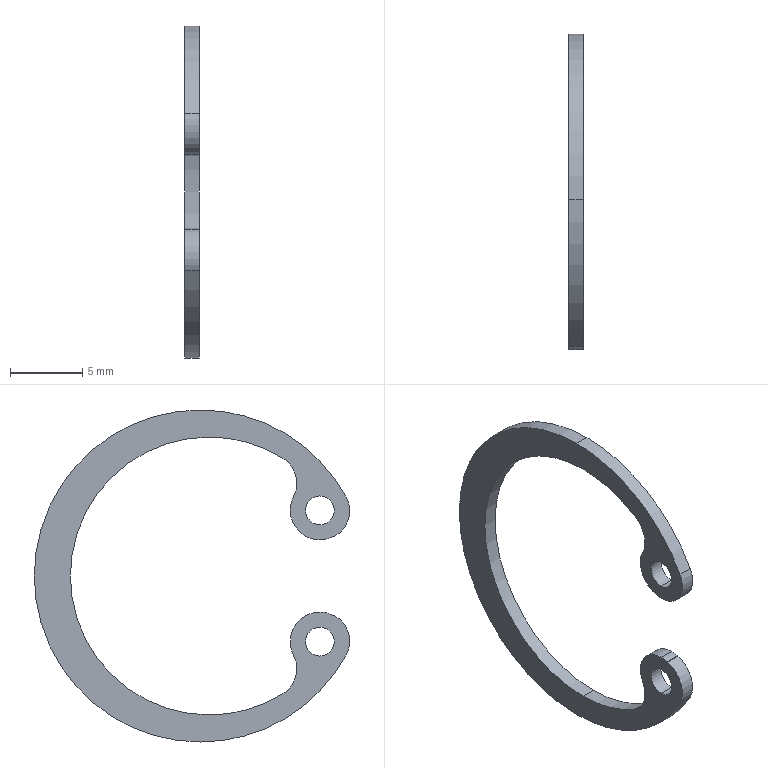Part | SolidWorks | features BaseBody 1 | 1 solid | 21 faces | box 1 x 21.856 x 23 mm | volume 128.626 mm3 | cylinder 17 | plane 4 | commonest cylinder face diameters 4.1 x5 2 x4 19.25 x3 23 x3 4 x2
STEP:
#1=CARTESIAN_POINT('',(-0.5,-8.916,-2.599));
#2=VERTEX_POINT('',#1);
#3=CARTESIAN_POINT('',(-0.5,-10.115,-5.471));
#4=VERTEX_POINT('',#3);
#5=CARTESIAN_POINT('',(-0.5,-8.356,-4.519));
#6=DIRECTION('',(1.,0.,0.));
#7=DIRECTION('',(0.,0.,-1.));
#8=AXIS2_PLACEMENT_3D('',#5,#6,#7);
#9=CIRCLE('',#8,2.);
#10=EDGE_CURVE('',#2,#4,#9,.T.);
#11=ORIENTED_EDGE('',*,*,#10,.T.);
#12=CARTESIAN_POINT('',(0.5,-10.115,-5.471));
#13=VERTEX_POINT('',#12);
#14=CARTESIAN_POINT('',(0.5,-10.115,-5.471));
#15=DIRECTION('',(-1.,0.,0.));
#16=VECTOR('',#15,1000.);
#17=LINE('',#14,#16);
#18=EDGE_CURVE('',#13,#4,#17,.T.);
#19=ORIENTED_EDGE('',*,*,#18,.F.);
#20=CARTESIAN_POINT('',(0.5,-8.916,-2.599));
#21=VERTEX_POINT('',#20);
#22=CARTESIAN_POINT('',(0.5,-8.356,-4.519));
#23=DIRECTION('',(1.,0.,0.));
#24=DIRECTION('',(0.,0.,-1.));
#25=AXIS2_PLACEMENT_3D('',#22,#23,#24);
#26=CIRCLE('',#25,2.);
#27=EDGE_CURVE('',#21,#13,#26,.T.);
#28=ORIENTED_EDGE('',*,*,#27,.F.);
#29=CARTESIAN_POINT('',(0.5,-8.916,-2.599));
#30=DIRECTION('',(-1.,0.,0.));
#31=VECTOR('',#30,1000.);
#32=LINE('',#29,#31);
#33=EDGE_CURVE('',#21,#2,#32,.T.);
#34=ORIENTED_EDGE('',*,*,#33,.T.);
#35=EDGE_LOOP('',(#11,#19,#28,#34));
#36=FACE_OUTER_BOUND('',#35,.T.);
#37=CARTESIAN_POINT('',(0.5,-8.356,-4.519));
#38=DIRECTION('',(-1.,0.,0.));
#39=DIRECTION('',(0.,0.,1.));
#40=AXIS2_PLACEMENT_3D('',#37,#38,#39);
#41=CYLINDRICAL_SURFACE('',#40,2.);
#42=ADVANCED_FACE('',(#36),#41,.T.);
#43=CARTESIAN_POINT('',(0.5,0.,-11.5));
#44=VERTEX_POINT('',#43);
#45=CARTESIAN_POINT('',(-0.5,0.,-11.5));
#46=VERTEX_POINT('',#45);
#47=CARTESIAN_POINT('',(0.5,0.,-11.5));
#48=DIRECTION('',(-1.,0.,0.));
#49=VECTOR('',#48,1000.);
#50=LINE('',#47,#49);
#51=EDGE_CURVE('',#44,#46,#50,.T.);
#52=ORIENTED_EDGE('',*,*,#51,.F.);
#53=CARTESIAN_POINT('',(0.5,0.,0.));
#54=DIRECTION('',(1.,0.,0.));
#55=DIRECTION('',(0.,0.,-1.));
#56=AXIS2_PLACEMENT_3D('',#53,#54,#55);
#57=CIRCLE('',#56,11.5);
#58=EDGE_CURVE('',#13,#44,#57,.T.);
#59=ORIENTED_EDGE('',*,*,#58,.F.);
#60=ORIENTED_EDGE('',*,*,#18,.T.);
#61=CARTESIAN_POINT('',(-0.5,0.,0.));
#62=DIRECTION('',(1.,0.,0.));
#63=DIRECTION('',(0.,0.,-1.));
#64=AXIS2_PLACEMENT_3D('',#61,#62,#63);
#65=CIRCLE('',#64,11.5);
#66=EDGE_CURVE('',#4,#46,#65,.T.);
#67=ORIENTED_EDGE('',*,*,#66,.T.);
#68=EDGE_LOOP('',(#52,#59,#60,#67));
#69=FACE_OUTER_BOUND('',#68,.T.);
#70=CARTESIAN_POINT('',(0.5,0.,0.));
#71=DIRECTION('',(-1.,0.,0.));
#72=DIRECTION('',(0.,0.,1.));
#73=AXIS2_PLACEMENT_3D('',#70,#71,#72);
#74=CYLINDRICAL_SURFACE('',#73,11.5);
#75=ADVANCED_FACE('',(#69),#74,.T.);
#76=CARTESIAN_POINT('',(-0.5,-10.115,5.471));
#77=VERTEX_POINT('',#76);
#78=CARTESIAN_POINT('',(-0.5,-8.916,2.599));
#79=VERTEX_POINT('',#78);
#80=CARTESIAN_POINT('',(-0.5,-8.356,4.519));
#81=DIRECTION('',(1.,0.,0.));
#82=DIRECTION('',(0.,0.,-1.));
#83=AXIS2_PLACEMENT_3D('',#80,#81,#82);
#84=CIRCLE('',#83,2.);
#85=EDGE_CURVE('',#77,#79,#84,.T.);
#86=ORIENTED_EDGE('',*,*,#85,.T.);
#87=CARTESIAN_POINT('',(0.5,-8.916,2.599));
#88=VERTEX_POINT('',#87);
#89=CARTESIAN_POINT('',(0.5,-8.916,2.599));
#90=DIRECTION('',(-1.,0.,0.));
#91=VECTOR('',#90,1000.);
#92=LINE('',#89,#91);
#93=EDGE_CURVE('',#88,#79,#92,.T.);
#94=ORIENTED_EDGE('',*,*,#93,.F.);
#95=CARTESIAN_POINT('',(0.5,-10.115,5.471));
#96=VERTEX_POINT('',#95);
#97=CARTESIAN_POINT('',(0.5,-8.356,4.519));
#98=DIRECTION('',(1.,0.,0.));
#99=DIRECTION('',(0.,0.,-1.));
#100=AXIS2_PLACEMENT_3D('',#97,#98,#99);
#101=CIRCLE('',#100,2.);
#102=EDGE_CURVE('',#96,#88,#101,.T.);
#103=ORIENTED_EDGE('',*,*,#102,.F.);
#104=CARTESIAN_POINT('',(0.5,-10.115,5.471));
#105=DIRECTION('',(-1.,0.,0.));
#106=VECTOR('',#105,1000.);
#107=LINE('',#104,#106);
#108=EDGE_CURVE('',#96,#77,#107,.T.);
#109=ORIENTED_EDGE('',*,*,#108,.T.);
#110=EDGE_LOOP('',(#86,#94,#103,#109));
#111=FACE_OUTER_BOUND('',#110,.T.);
#112=CARTESIAN_POINT('',(0.5,-8.356,4.519));
#113=DIRECTION('',(-1.,0.,0.));
#114=DIRECTION('',(0.,0.,1.));
#115=AXIS2_PLACEMENT_3D('',#112,#113,#114);
#116=CYLINDRICAL_SURFACE('',#115,2.);
#117=ADVANCED_FACE('',(#111),#116,.T.);
#118=CARTESIAN_POINT('',(-0.5,-8.856,2.582));
#119=VERTEX_POINT('',#118);
#120=CARTESIAN_POINT('',(-0.5,-8.916,2.599));
#121=DIRECTION('',(0.,0.96,-0.2799));
#122=VECTOR('',#121,1000.);
#123=LINE('',#120,#122);
#124=EDGE_CURVE('',#79,#119,#123,.T.);
#125=ORIENTED_EDGE('',*,*,#124,.T.);
#126=CARTESIAN_POINT('',(0.5,-8.856,2.582));
#127=VERTEX_POINT('',#126);
#128=CARTESIAN_POINT('',(0.5,-8.856,2.582));
#129=DIRECTION('',(-1.,0.,0.));
#130=VECTOR('',#129,1000.);
#131=LINE('',#128,#130);
#132=EDGE_CURVE('',#127,#119,#131,.T.);
#133=ORIENTED_EDGE('',*,*,#132,.F.);
#134=CARTESIAN_POINT('',(0.5,-8.916,2.599));
#135=DIRECTION('',(0.,0.96,-0.2799));
#136=VECTOR('',#135,1000.);
#137=LINE('',#134,#136);
#138=EDGE_CURVE('',#88,#127,#137,.T.);
#139=ORIENTED_EDGE('',*,*,#138,.F.);
#140=ORIENTED_EDGE('',*,*,#93,.T.);
#141=EDGE_LOOP('',(#125,#133,#139,#140));
#142=FACE_OUTER_BOUND('',#141,.T.);
#143=CARTESIAN_POINT('',(0.5,-8.916,2.599));
#144=DIRECTION('',(0.,0.2799,0.96));
#145=DIRECTION('',(1.,0.,0.));
#146=AXIS2_PLACEMENT_3D('',#143,#144,#145);
#147=PLANE('',#146);
#148=ADVANCED_FACE('',(#142),#147,.F.);
#149=CARTESIAN_POINT('',(-0.5,-6.46,5.488));
#150=VERTEX_POINT('',#149);
#151=CARTESIAN_POINT('',(-0.5,-8.283,4.55));
#152=DIRECTION('',(1.,0.,0.));
#153=DIRECTION('',(0.,0.,-1.));
#154=AXIS2_PLACEMENT_3D('',#151,#152,#153);
#155=CIRCLE('',#154,2.05);
#156=EDGE_CURVE('',#119,#150,#155,.T.);
#157=ORIENTED_EDGE('',*,*,#156,.T.);
#158=CARTESIAN_POINT('',(0.5,-6.46,5.488));
#159=VERTEX_POINT('',#158);
#160=CARTESIAN_POINT('',(0.5,-6.46,5.488));
#161=DIRECTION('',(-1.,0.,0.));
#162=VECTOR('',#161,1000.);
#163=LINE('',#160,#162);
#164=EDGE_CURVE('',#159,#150,#163,.T.);
#165=ORIENTED_EDGE('',*,*,#164,.F.);
#166=CARTESIAN_POINT('',(0.5,-8.283,4.55));
#167=DIRECTION('',(1.,0.,0.));
#168=DIRECTION('',(0.,0.,-1.));
#169=AXIS2_PLACEMENT_3D('',#166,#167,#168);
#170=CIRCLE('',#169,2.05);
#171=EDGE_CURVE('',#127,#159,#170,.T.);
#172=ORIENTED_EDGE('',*,*,#171,.F.);
#173=ORIENTED_EDGE('',*,*,#132,.T.);
#174=EDGE_LOOP('',(#157,#165,#172,#173));
#175=FACE_OUTER_BOUND('',#174,.T.);
#176=CARTESIAN_POINT('',(0.5,-8.283,4.55));
#177=DIRECTION('',(-1.,0.,0.));
#178=DIRECTION('',(0.,0.,1.));
#179=AXIS2_PLACEMENT_3D('',#176,#177,#178);
#180=CYLINDRICAL_SURFACE('',#179,2.05);
#181=ADVANCED_FACE('',(#175),#180,.T.);
#182=CARTESIAN_POINT('',(-0.5,-5.722,8.164));
#183=VERTEX_POINT('',#182);
#184=CARTESIAN_POINT('',(-0.5,-4.637,6.426));
#185=DIRECTION('',(1.,0.,0.));
#186=DIRECTION('',(0.,0.,-1.));
#187=AXIS2_PLACEMENT_3D('',#184,#185,#186);
#188=CIRCLE('',#187,2.05);
#189=EDGE_CURVE('',#183,#150,#188,.T.);
#190=ORIENTED_EDGE('',*,*,#189,.F.);
#191=CARTESIAN_POINT('',(0.5,-5.722,8.164));
#192=VERTEX_POINT('',#191);
#193=CARTESIAN_POINT('',(0.5,-5.722,8.164));
#194=DIRECTION('',(-1.,0.,0.));
#195=VECTOR('',#194,1000.);
#196=LINE('',#193,#195);
#197=EDGE_CURVE('',#192,#183,#196,.T.);
#198=ORIENTED_EDGE('',*,*,#197,.F.);
#199=CARTESIAN_POINT('',(0.5,-4.637,6.426));
#200=DIRECTION('',(1.,0.,0.));
#201=DIRECTION('',(0.,0.,-1.));
#202=AXIS2_PLACEMENT_3D('',#199,#200,#201);
#203=CIRCLE('',#202,2.05);
#204=EDGE_CURVE('',#192,#159,#203,.T.);
#205=ORIENTED_EDGE('',*,*,#204,.T.);
#206=ORIENTED_EDGE('',*,*,#164,.T.);
#207=EDGE_LOOP('',(#190,#198,#205,#206));
#208=FACE_OUTER_BOUND('',#207,.T.);
#209=CARTESIAN_POINT('',(0.5,-4.637,6.426));
#210=DIRECTION('',(-1.,0.,0.));
#211=DIRECTION('',(0.,0.,1.));
#212=AXIS2_PLACEMENT_3D('',#209,#210,#211);
#213=CYLINDRICAL_SURFACE('',#212,2.05);
#214=ADVANCED_FACE('',(#208),#213,.F.);
#215=CARTESIAN_POINT('',(0.5,-0.625,9.625));
#216=VERTEX_POINT('',#215);
#217=CARTESIAN_POINT('',(-0.5,-0.625,9.625));
#218=VERTEX_POINT('',#217);
#219=CARTESIAN_POINT('',(0.5,-0.625,9.625));
#220=DIRECTION('',(-1.,0.,0.));
#221=VECTOR('',#220,1000.);
#222=LINE('',#219,#221);
#223=EDGE_CURVE('',#216,#218,#222,.T.);
#224=ORIENTED_EDGE('',*,*,#223,.F.);
#225=CARTESIAN_POINT('',(0.5,-0.625,0.));
#226=DIRECTION('',(1.,0.,0.));
#227=DIRECTION('',(0.,0.,-1.));
#228=AXIS2_PLACEMENT_3D('',#225,#226,#227);
#229=CIRCLE('',#228,9.625);
#230=EDGE_CURVE('',#216,#192,#229,.T.);
#231=ORIENTED_EDGE('',*,*,#230,.T.);
#232=ORIENTED_EDGE('',*,*,#197,.T.);
#233=CARTESIAN_POINT('',(-0.5,-0.625,0.));
#234=DIRECTION('',(1.,0.,0.));
#235=DIRECTION('',(0.,0.,-1.));
#236=AXIS2_PLACEMENT_3D('',#233,#234,#235);
#237=CIRCLE('',#236,9.625);
#238=EDGE_CURVE('',#218,#183,#237,.T.);
#239=ORIENTED_EDGE('',*,*,#238,.F.);
#240=EDGE_LOOP('',(#224,#231,#232,#239));
#241=FACE_OUTER_BOUND('',#240,.T.);
#242=CARTESIAN_POINT('',(0.5,-0.625,0.));
#243=DIRECTION('',(-1.,0.,0.));
#244=DIRECTION('',(0.,0.,1.));
#245=AXIS2_PLACEMENT_3D('',#242,#243,#244);
#246=CYLINDRICAL_SURFACE('',#245,9.625);
#247=ADVANCED_FACE('',(#241),#246,.F.);
#248=CARTESIAN_POINT('',(-0.5,-6.46,-5.488));
#249=VERTEX_POINT('',#248);
#250=CARTESIAN_POINT('',(-0.5,-5.722,-8.164));
#251=VERTEX_POINT('',#250);
#252=CARTESIAN_POINT('',(-0.5,-4.637,-6.426));
#253=DIRECTION('',(1.,0.,0.));
#254=DIRECTION('',(0.,0.,-1.));
#255=AXIS2_PLACEMENT_3D('',#252,#253,#254);
#256=CIRCLE('',#255,2.05);
#257=EDGE_CURVE('',#249,#251,#256,.T.);
#258=ORIENTED_EDGE('',*,*,#257,.F.);
#259=CARTESIAN_POINT('',(0.5,-6.46,-5.488));
#260=VERTEX_POINT('',#259);
#261=CARTESIAN_POINT('',(0.5,-6.46,-5.488));
#262=DIRECTION('',(-1.,0.,0.));
#263=VECTOR('',#262,1000.);
#264=LINE('',#261,#263);
#265=EDGE_CURVE('',#260,#249,#264,.T.);
#266=ORIENTED_EDGE('',*,*,#265,.F.);
#267=CARTESIAN_POINT('',(0.5,-5.722,-8.164));
#268=VERTEX_POINT('',#267);
#269=CARTESIAN_POINT('',(0.5,-4.637,-6.426));
#270=DIRECTION('',(1.,0.,0.));
#271=DIRECTION('',(0.,0.,-1.));
#272=AXIS2_PLACEMENT_3D('',#269,#270,#271);
#273=CIRCLE('',#272,2.05);
#274=EDGE_CURVE('',#260,#268,#273,.T.);
#275=ORIENTED_EDGE('',*,*,#274,.T.);
#276=CARTESIAN_POINT('',(0.5,-5.722,-8.164));
#277=DIRECTION('',(-1.,0.,0.));
#278=VECTOR('',#277,1000.);
#279=LINE('',#276,#278);
#280=EDGE_CURVE('',#268,#251,#279,.T.);
#281=ORIENTED_EDGE('',*,*,#280,.T.);
#282=EDGE_LOOP('',(#258,#266,#275,#281));
#283=FACE_OUTER_BOUND('',#282,.T.);
#284=CARTESIAN_POINT('',(0.5,-4.637,-6.426));
#285=DIRECTION('',(-1.,0.,0.));
#286=DIRECTION('',(0.,0.,1.));
#287=AXIS2_PLACEMENT_3D('',#284,#285,#286);
#288=CYLINDRICAL_SURFACE('',#287,2.05);
#289=ADVANCED_FACE('',(#283),#288,.F.);
#290=CARTESIAN_POINT('',(0.5,-8.283,-2.5));
#291=VERTEX_POINT('',#290);
#292=CARTESIAN_POINT('',(-0.5,-8.283,-2.5));
#293=VERTEX_POINT('',#292);
#294=CARTESIAN_POINT('',(0.5,-8.283,-2.5));
#295=DIRECTION('',(-1.,0.,0.));
#296=VECTOR('',#295,1000.);
#297=LINE('',#294,#296);
#298=EDGE_CURVE('',#291,#293,#297,.T.);
#299=ORIENTED_EDGE('',*,*,#298,.F.);
#300=CARTESIAN_POINT('',(0.5,-8.283,-4.55));
#301=DIRECTION('',(1.,0.,0.));
#302=DIRECTION('',(0.,0.,-1.));
#303=AXIS2_PLACEMENT_3D('',#300,#301,#302);
#304=CIRCLE('',#303,2.05);
#305=EDGE_CURVE('',#260,#291,#304,.T.);
#306=ORIENTED_EDGE('',*,*,#305,.F.);
#307=ORIENTED_EDGE('',*,*,#265,.T.);
#308=CARTESIAN_POINT('',(-0.5,-8.283,-4.55));
#309=DIRECTION('',(1.,0.,0.));
#310=DIRECTION('',(0.,0.,-1.));
#311=AXIS2_PLACEMENT_3D('',#308,#309,#310);
#312=CIRCLE('',#311,2.05);
#313=EDGE_CURVE('',#249,#293,#312,.T.);
#314=ORIENTED_EDGE('',*,*,#313,.T.);
#315=EDGE_LOOP('',(#299,#306,#307,#314));
#316=FACE_OUTER_BOUND('',#315,.T.);
#317=CARTESIAN_POINT('',(0.5,-8.283,-4.55));
#318=DIRECTION('',(-1.,0.,0.));
#319=DIRECTION('',(0.,0.,1.));
#320=AXIS2_PLACEMENT_3D('',#317,#318,#319);
#321=CYLINDRICAL_SURFACE('',#320,2.05);
#322=ADVANCED_FACE('',(#316),#321,.T.);
#323=CARTESIAN_POINT('',(0.5,-8.283,-5.55));
#324=VERTEX_POINT('',#323);
#325=CARTESIAN_POINT('',(-0.5,-8.283,-5.55));
#326=VERTEX_POINT('',#325);
#327=CARTESIAN_POINT('',(0.5,-8.283,-5.55));
#328=DIRECTION('',(-1.,0.,0.));
#329=VECTOR('',#328,1000.);
#330=LINE('',#327,#329);
#331=EDGE_CURVE('',#324,#326,#330,.T.);
#332=ORIENTED_EDGE('',*,*,#331,.F.);
#333=CARTESIAN_POINT('',(0.5,-8.283,-3.55));
#334=VERTEX_POINT('',#333);
#335=CARTESIAN_POINT('',(0.5,-8.283,-4.55));
#336=DIRECTION('',(1.,0.,0.));
#337=DIRECTION('',(0.,0.,-1.));
#338=AXIS2_PLACEMENT_3D('',#335,#336,#337);
#339=CIRCLE('',#338,1.);
#340=EDGE_CURVE('',#324,#334,#339,.T.);
#341=ORIENTED_EDGE('',*,*,#340,.T.);
#342=CARTESIAN_POINT('',(-0.5,-8.283,-3.55));
#343=VERTEX_POINT('',#342);
#344=CARTESIAN_POINT('',(0.5,-8.283,-3.55));
#345=DIRECTION('',(-1.,0.,0.));
#346=VECTOR('',#345,1000.);
#347=LINE('',#344,#346);
#348=EDGE_CURVE('',#334,#343,#347,.T.);
#349=ORIENTED_EDGE('',*,*,#348,.T.);
#350=CARTESIAN_POINT('',(-0.5,-8.283,-4.55));
#351=DIRECTION('',(1.,0.,0.));
#352=DIRECTION('',(0.,0.,-1.));
#353=AXIS2_PLACEMENT_3D('',#350,#351,#352);
#354=CIRCLE('',#353,1.);
#355=EDGE_CURVE('',#326,#343,#354,.T.);
#356=ORIENTED_EDGE('',*,*,#355,.F.);
#357=EDGE_LOOP('',(#332,#341,#349,#356));
#358=FACE_OUTER_BOUND('',#357,.T.);
#359=CARTESIAN_POINT('',(0.5,-8.283,-4.55));
#360=DIRECTION('',(-1.,0.,0.));
#361=DIRECTION('',(0.,0.,1.));
#362=AXIS2_PLACEMENT_3D('',#359,#360,#361);
#363=CYLINDRICAL_SURFACE('',#362,1.);
#364=ADVANCED_FACE('',(#358),#363,.F.);
#365=CARTESIAN_POINT('',(0.5,-8.283,3.55));
#366=VERTEX_POINT('',#365);
#367=CARTESIAN_POINT('',(-0.5,-8.283,3.55));
#368=VERTEX_POINT('',#367);
#369=CARTESIAN_POINT('',(0.5,-8.283,3.55));
#370=DIRECTION('',(-1.,0.,0.));
#371=VECTOR('',#370,1000.);
#372=LINE('',#369,#371);
#373=EDGE_CURVE('',#366,#368,#372,.T.);
#374=ORIENTED_EDGE('',*,*,#373,.F.);
#375=CARTESIAN_POINT('',(0.5,-8.283,5.55));
#376=VERTEX_POINT('',#375);
#377=CARTESIAN_POINT('',(0.5,-8.283,4.55));
#378=DIRECTION('',(1.,0.,0.));
#379=DIRECTION('',(0.,0.,-1.));
#380=AXIS2_PLACEMENT_3D('',#377,#378,#379);
#381=CIRCLE('',#380,1.);
#382=EDGE_CURVE('',#366,#376,#381,.T.);
#383=ORIENTED_EDGE('',*,*,#382,.T.);
#384=CARTESIAN_POINT('',(-0.5,-8.283,5.55));
#385=VERTEX_POINT('',#384);
#386=CARTESIAN_POINT('',(0.5,-8.283,5.55));
#387=DIRECTION('',(-1.,0.,0.));
#388=VECTOR('',#387,1000.);
#389=LINE('',#386,#388);
#390=EDGE_CURVE('',#376,#385,#389,.T.);
#391=ORIENTED_EDGE('',*,*,#390,.T.);
#392=CARTESIAN_POINT('',(-0.5,-8.283,4.55));
#393=DIRECTION('',(1.,0.,0.));
#394=DIRECTION('',(0.,0.,-1.));
#395=AXIS2_PLACEMENT_3D('',#392,#393,#394);
#396=CIRCLE('',#395,1.);
#397=EDGE_CURVE('',#368,#385,#396,.T.);
#398=ORIENTED_EDGE('',*,*,#397,.F.);
#399=EDGE_LOOP('',(#374,#383,#391,#398));
#400=FACE_OUTER_BOUND('',#399,.T.);
#401=CARTESIAN_POINT('',(0.5,-8.283,4.55));
#402=DIRECTION('',(-1.,0.,0.));
#403=DIRECTION('',(0.,0.,1.));
#404=AXIS2_PLACEMENT_3D('',#401,#402,#403);
#405=CYLINDRICAL_SURFACE('',#404,1.);
#406=ADVANCED_FACE('',(#400),#405,.F.);
#407=CARTESIAN_POINT('',(-0.5,-8.856,-2.582));
#408=VERTEX_POINT('',#407);
#409=CARTESIAN_POINT('',(-0.5,-8.856,-2.582));
#410=DIRECTION('',(0.,-0.96,-0.2799));
#411=VECTOR('',#410,1000.);
#412=LINE('',#409,#411);
#413=EDGE_CURVE('',#408,#2,#412,.T.);
#414=ORIENTED_EDGE('',*,*,#413,.T.);
#415=ORIENTED_EDGE('',*,*,#33,.F.);
#416=CARTESIAN_POINT('',(0.5,-8.856,-2.582));
#417=VERTEX_POINT('',#416);
#418=CARTESIAN_POINT('',(0.5,-8.856,-2.582));
#419=DIRECTION('',(0.,-0.96,-0.2799));
#420=VECTOR('',#419,1000.);
#421=LINE('',#418,#420);
#422=EDGE_CURVE('',#417,#21,#421,.T.);
#423=ORIENTED_EDGE('',*,*,#422,.F.);
#424=CARTESIAN_POINT('',(0.5,-8.856,-2.582));
#425=DIRECTION('',(-1.,0.,0.));
#426=VECTOR('',#425,1000.);
#427=LINE('',#424,#426);
#428=EDGE_CURVE('',#417,#408,#427,.T.);
#429=ORIENTED_EDGE('',*,*,#428,.T.);
#430=EDGE_LOOP('',(#414,#415,#423,#429));
#431=FACE_OUTER_BOUND('',#430,.T.);
#432=CARTESIAN_POINT('',(0.5,-8.856,-2.582));
#433=DIRECTION('',(0.,0.2799,-0.96));
#434=DIRECTION('',(-1.,0.,0.));
#435=AXIS2_PLACEMENT_3D('',#432,#433,#434);
#436=PLANE('',#435);
#437=ADVANCED_FACE('',(#431),#436,.F.);
#438=CARTESIAN_POINT('',(0.5,-8.283,4.55));
#439=DIRECTION('',(1.,0.,0.));
#440=DIRECTION('',(0.,0.,-1.));
#441=AXIS2_PLACEMENT_3D('',#438,#439,#440);
#442=CIRCLE('',#441,1.);
#443=EDGE_CURVE('',#376,#366,#442,.T.);
#444=ORIENTED_EDGE('',*,*,#443,.F.);
#445=ORIENTED_EDGE('',*,*,#382,.F.);
#446=EDGE_LOOP('',(#444,#445));
#447=FACE_BOUND('',#446,.T.);
#448=CARTESIAN_POINT('',(0.5,-8.283,-4.55));
#449=DIRECTION('',(1.,0.,0.));
#450=DIRECTION('',(0.,0.,-1.));
#451=AXIS2_PLACEMENT_3D('',#448,#449,#450);
#452=CIRCLE('',#451,1.);
#453=EDGE_CURVE('',#334,#324,#452,.T.);
#454=ORIENTED_EDGE('',*,*,#453,.F.);
#455=ORIENTED_EDGE('',*,*,#340,.F.);
#456=EDGE_LOOP('',(#454,#455));
#457=FACE_BOUND('',#456,.T.);
#458=ORIENTED_EDGE('',*,*,#27,.T.);
#459=ORIENTED_EDGE('',*,*,#58,.T.);
#460=CARTESIAN_POINT('',(0.5,0.,11.5));
#461=VERTEX_POINT('',#460);
#462=CARTESIAN_POINT('',(0.5,0.,0.));
#463=DIRECTION('',(1.,0.,0.));
#464=DIRECTION('',(0.,0.,-1.));
#465=AXIS2_PLACEMENT_3D('',#462,#463,#464);
#466=CIRCLE('',#465,11.5);
#467=EDGE_CURVE('',#44,#461,#466,.T.);
#468=ORIENTED_EDGE('',*,*,#467,.T.);
#469=CARTESIAN_POINT('',(0.5,0.,0.));
#470=DIRECTION('',(1.,0.,0.));
#471=DIRECTION('',(0.,0.,-1.));
#472=AXIS2_PLACEMENT_3D('',#469,#470,#471);
#473=CIRCLE('',#472,11.5);
#474=EDGE_CURVE('',#461,#96,#473,.T.);
#475=ORIENTED_EDGE('',*,*,#474,.T.);
#476=ORIENTED_EDGE('',*,*,#102,.T.);
#477=ORIENTED_EDGE('',*,*,#138,.T.);
#478=ORIENTED_EDGE('',*,*,#171,.T.);
#479=ORIENTED_EDGE('',*,*,#204,.F.);
#480=ORIENTED_EDGE('',*,*,#230,.F.);
#481=CARTESIAN_POINT('',(0.5,-0.625,-9.625));
#482=VERTEX_POINT('',#481);
#483=CARTESIAN_POINT('',(0.5,-0.625,0.));
#484=DIRECTION('',(1.,0.,0.));
#485=DIRECTION('',(0.,0.,-1.));
#486=AXIS2_PLACEMENT_3D('',#483,#484,#485);
#487=CIRCLE('',#486,9.625);
#488=EDGE_CURVE('',#482,#216,#487,.T.);
#489=ORIENTED_EDGE('',*,*,#488,.F.);
#490=CARTESIAN_POINT('',(0.5,-0.625,0.));
#491=DIRECTION('',(1.,0.,0.));
#492=DIRECTION('',(0.,0.,-1.));
#493=AXIS2_PLACEMENT_3D('',#490,#491,#492);
#494=CIRCLE('',#493,9.625);
#495=EDGE_CURVE('',#268,#482,#494,.T.);
#496=ORIENTED_EDGE('',*,*,#495,.F.);
#497=ORIENTED_EDGE('',*,*,#274,.F.);
#498=ORIENTED_EDGE('',*,*,#305,.T.);
#499=CARTESIAN_POINT('',(0.5,-8.283,-4.55));
#500=DIRECTION('',(1.,0.,0.));
#501=DIRECTION('',(0.,0.,-1.));
#502=AXIS2_PLACEMENT_3D('',#499,#500,#501);
#503=CIRCLE('',#502,2.05);
#504=EDGE_CURVE('',#291,#417,#503,.T.);
#505=ORIENTED_EDGE('',*,*,#504,.T.);
#506=ORIENTED_EDGE('',*,*,#422,.T.);
#507=EDGE_LOOP('',(#458,#459,#468,#475,#476,#477,#478,#479,#480,#489,#496,#497,#498,#505,#506));
#508=FACE_OUTER_BOUND('',#507,.T.);
#509=CARTESIAN_POINT('',(0.5,-8.356,-4.519));
#510=DIRECTION('',(1.,0.,0.));
#511=DIRECTION('',(0.,1.,0.));
#512=AXIS2_PLACEMENT_3D('',#509,#510,#511);
#513=PLANE('',#512);
#514=ADVANCED_FACE('',(#447,#457,#508),#513,.T.);
#515=CARTESIAN_POINT('',(-0.5,-8.283,4.55));
#516=DIRECTION('',(1.,0.,0.));
#517=DIRECTION('',(0.,0.,-1.));
#518=AXIS2_PLACEMENT_3D('',#515,#516,#517);
#519=CIRCLE('',#518,1.);
#520=EDGE_CURVE('',#385,#368,#519,.T.);
#521=ORIENTED_EDGE('',*,*,#520,.T.);
#522=ORIENTED_EDGE('',*,*,#397,.T.);
#523=EDGE_LOOP('',(#521,#522));
#524=FACE_BOUND('',#523,.T.);
#525=CARTESIAN_POINT('',(-0.5,-8.283,-4.55));
#526=DIRECTION('',(1.,0.,0.));
#527=DIRECTION('',(0.,0.,-1.));
#528=AXIS2_PLACEMENT_3D('',#525,#526,#527);
#529=CIRCLE('',#528,1.);
#530=EDGE_CURVE('',#343,#326,#529,.T.);
#531=ORIENTED_EDGE('',*,*,#530,.T.);
#532=ORIENTED_EDGE('',*,*,#355,.T.);
#533=EDGE_LOOP('',(#531,#532));
#534=FACE_BOUND('',#533,.T.);
#535=ORIENTED_EDGE('',*,*,#10,.F.);
#536=ORIENTED_EDGE('',*,*,#413,.F.);
#537=CARTESIAN_POINT('',(-0.5,-8.283,-4.55));
#538=DIRECTION('',(1.,0.,0.));
#539=DIRECTION('',(0.,0.,-1.));
#540=AXIS2_PLACEMENT_3D('',#537,#538,#539);
#541=CIRCLE('',#540,2.05);
#542=EDGE_CURVE('',#293,#408,#541,.T.);
#543=ORIENTED_EDGE('',*,*,#542,.F.);
#544=ORIENTED_EDGE('',*,*,#313,.F.);
#545=ORIENTED_EDGE('',*,*,#257,.T.);
#546=CARTESIAN_POINT('',(-0.5,-0.625,-9.625));
#547=VERTEX_POINT('',#546);
#548=CARTESIAN_POINT('',(-0.5,-0.625,0.));
#549=DIRECTION('',(1.,0.,0.));
#550=DIRECTION('',(0.,0.,-1.));
#551=AXIS2_PLACEMENT_3D('',#548,#549,#550);
#552=CIRCLE('',#551,9.625);
#553=EDGE_CURVE('',#251,#547,#552,.T.);
#554=ORIENTED_EDGE('',*,*,#553,.T.);
#555=CARTESIAN_POINT('',(-0.5,-0.625,0.));
#556=DIRECTION('',(1.,0.,0.));
#557=DIRECTION('',(0.,0.,-1.));
#558=AXIS2_PLACEMENT_3D('',#555,#556,#557);
#559=CIRCLE('',#558,9.625);
#560=EDGE_CURVE('',#547,#218,#559,.T.);
#561=ORIENTED_EDGE('',*,*,#560,.T.);
#562=ORIENTED_EDGE('',*,*,#238,.T.);
#563=ORIENTED_EDGE('',*,*,#189,.T.);
#564=ORIENTED_EDGE('',*,*,#156,.F.);
#565=ORIENTED_EDGE('',*,*,#124,.F.);
#566=ORIENTED_EDGE('',*,*,#85,.F.);
#567=CARTESIAN_POINT('',(-0.5,0.,11.5));
#568=VERTEX_POINT('',#567);
#569=CARTESIAN_POINT('',(-0.5,0.,0.));
#570=DIRECTION('',(1.,0.,0.));
#571=DIRECTION('',(0.,0.,-1.));
#572=AXIS2_PLACEMENT_3D('',#569,#570,#571);
#573=CIRCLE('',#572,11.5);
#574=EDGE_CURVE('',#568,#77,#573,.T.);
#575=ORIENTED_EDGE('',*,*,#574,.F.);
#576=CARTESIAN_POINT('',(-0.5,0.,0.));
#577=DIRECTION('',(1.,0.,0.));
#578=DIRECTION('',(0.,0.,-1.));
#579=AXIS2_PLACEMENT_3D('',#576,#577,#578);
#580=CIRCLE('',#579,11.5);
#581=EDGE_CURVE('',#46,#568,#580,.T.);
#582=ORIENTED_EDGE('',*,*,#581,.F.);
#583=ORIENTED_EDGE('',*,*,#66,.F.);
#584=EDGE_LOOP('',(#535,#536,#543,#544,#545,#554,#561,#562,#563,#564,#565,#566,#575,#582,#583));
#585=FACE_OUTER_BOUND('',#584,.T.);
#586=CARTESIAN_POINT('',(-0.5,-8.356,-4.519));
#587=DIRECTION('',(1.,0.,0.));
#588=DIRECTION('',(0.,1.,0.));
#589=AXIS2_PLACEMENT_3D('',#586,#587,#588);
#590=PLANE('',#589);
#591=ADVANCED_FACE('',(#524,#534,#585),#590,.F.);
#592=ORIENTED_EDGE('',*,*,#443,.T.);
#593=ORIENTED_EDGE('',*,*,#373,.T.);
#594=ORIENTED_EDGE('',*,*,#520,.F.);
#595=ORIENTED_EDGE('',*,*,#390,.F.);
#596=EDGE_LOOP('',(#592,#593,#594,#595));
#597=FACE_OUTER_BOUND('',#596,.T.);
#598=CARTESIAN_POINT('',(0.5,-8.283,4.55));
#599=DIRECTION('',(-1.,0.,0.));
#600=DIRECTION('',(0.,0.,1.));
#601=AXIS2_PLACEMENT_3D('',#598,#599,#600);
#602=CYLINDRICAL_SURFACE('',#601,1.);
#603=ADVANCED_FACE('',(#597),#602,.F.);
#604=ORIENTED_EDGE('',*,*,#453,.T.);
#605=ORIENTED_EDGE('',*,*,#331,.T.);
#606=ORIENTED_EDGE('',*,*,#530,.F.);
#607=ORIENTED_EDGE('',*,*,#348,.F.);
#608=EDGE_LOOP('',(#604,#605,#606,#607));
#609=FACE_OUTER_BOUND('',#608,.T.);
#610=CARTESIAN_POINT('',(0.5,-8.283,-4.55));
#611=DIRECTION('',(-1.,0.,0.));
#612=DIRECTION('',(0.,0.,1.));
#613=AXIS2_PLACEMENT_3D('',#610,#611,#612);
#614=CYLINDRICAL_SURFACE('',#613,1.);
#615=ADVANCED_FACE('',(#609),#614,.F.);
#616=ORIENTED_EDGE('',*,*,#504,.F.);
#617=ORIENTED_EDGE('',*,*,#298,.T.);
#618=ORIENTED_EDGE('',*,*,#542,.T.);
#619=ORIENTED_EDGE('',*,*,#428,.F.);
#620=EDGE_LOOP('',(#616,#617,#618,#619));
#621=FACE_OUTER_BOUND('',#620,.T.);
#622=CARTESIAN_POINT('',(0.5,-8.283,-4.55));
#623=DIRECTION('',(-1.,0.,0.));
#624=DIRECTION('',(0.,0.,1.));
#625=AXIS2_PLACEMENT_3D('',#622,#623,#624);
#626=CYLINDRICAL_SURFACE('',#625,2.05);
#627=ADVANCED_FACE('',(#621),#626,.T.);
#628=CARTESIAN_POINT('',(0.5,-0.625,-9.625));
#629=DIRECTION('',(-1.,0.,0.));
#630=VECTOR('',#629,1000.);
#631=LINE('',#628,#630);
#632=EDGE_CURVE('',#482,#547,#631,.T.);
#633=ORIENTED_EDGE('',*,*,#632,.F.);
#634=ORIENTED_EDGE('',*,*,#488,.T.);
#635=ORIENTED_EDGE('',*,*,#223,.T.);
#636=ORIENTED_EDGE('',*,*,#560,.F.);
#637=EDGE_LOOP('',(#633,#634,#635,#636));
#638=FACE_OUTER_BOUND('',#637,.T.);
#639=CARTESIAN_POINT('',(0.5,-0.625,0.));
#640=DIRECTION('',(-1.,0.,0.));
#641=DIRECTION('',(0.,0.,1.));
#642=AXIS2_PLACEMENT_3D('',#639,#640,#641);
#643=CYLINDRICAL_SURFACE('',#642,9.625);
#644=ADVANCED_FACE('',(#638),#643,.F.);
#645=ORIENTED_EDGE('',*,*,#495,.T.);
#646=ORIENTED_EDGE('',*,*,#632,.T.);
#647=ORIENTED_EDGE('',*,*,#553,.F.);
#648=ORIENTED_EDGE('',*,*,#280,.F.);
#649=EDGE_LOOP('',(#645,#646,#647,#648));
#650=FACE_OUTER_BOUND('',#649,.T.);
#651=CARTESIAN_POINT('',(0.5,-0.625,0.));
#652=DIRECTION('',(-1.,0.,0.));
#653=DIRECTION('',(0.,0.,1.));
#654=AXIS2_PLACEMENT_3D('',#651,#652,#653);
#655=CYLINDRICAL_SURFACE('',#654,9.625);
#656=ADVANCED_FACE('',(#650),#655,.F.);
#657=ORIENTED_EDGE('',*,*,#474,.F.);
#658=CARTESIAN_POINT('',(0.5,0.,11.5));
#659=DIRECTION('',(-1.,0.,0.));
#660=VECTOR('',#659,1000.);
#661=LINE('',#658,#660);
#662=EDGE_CURVE('',#461,#568,#661,.T.);
#663=ORIENTED_EDGE('',*,*,#662,.T.);
#664=ORIENTED_EDGE('',*,*,#574,.T.);
#665=ORIENTED_EDGE('',*,*,#108,.F.);
#666=EDGE_LOOP('',(#657,#663,#664,#665));
#667=FACE_OUTER_BOUND('',#666,.T.);
#668=CARTESIAN_POINT('',(0.5,0.,0.));
#669=DIRECTION('',(-1.,0.,0.));
#670=DIRECTION('',(0.,0.,1.));
#671=AXIS2_PLACEMENT_3D('',#668,#669,#670);
#672=CYLINDRICAL_SURFACE('',#671,11.5);
#673=ADVANCED_FACE('',(#667),#672,.T.);
#674=ORIENTED_EDGE('',*,*,#467,.F.);
#675=ORIENTED_EDGE('',*,*,#51,.T.);
#676=ORIENTED_EDGE('',*,*,#581,.T.);
#677=ORIENTED_EDGE('',*,*,#662,.F.);
#678=EDGE_LOOP('',(#674,#675,#676,#677));
#679=FACE_OUTER_BOUND('',#678,.T.);
#680=CARTESIAN_POINT('',(0.5,0.,0.));
#681=DIRECTION('',(-1.,0.,0.));
#682=DIRECTION('',(0.,0.,1.));
#683=AXIS2_PLACEMENT_3D('',#680,#681,#682);
#684=CYLINDRICAL_SURFACE('',#683,11.5);
#685=ADVANCED_FACE('',(#679),#684,.T.);
#686=CLOSED_SHELL('',(#42,#75,#117,#148,#181,#214,#247,#289,#322,#364,#406,#437,#514,#591,#603,#615,#627,#644,#656,#673,#685));
#687=MANIFOLD_SOLID_BREP('',#686);
#688=CARTESIAN_POINT('',(0.,0.,0.));
#689=DIRECTION('',(0.,0.,1.));
#690=DIRECTION('',(1.,0.,0.));
#691=AXIS2_PLACEMENT_3D('',#688,#689,#690);
#692=(LENGTH_UNIT()NAMED_UNIT(*)SI_UNIT(.MILLI.,.METRE.));
#693=UNCERTAINTY_MEASURE_WITH_UNIT(LENGTH_MEASURE(0.00001),#692,'','');
#694=(NAMED_UNIT(*)PLANE_ANGLE_UNIT()SI_UNIT($,.RADIAN.));
#695=(NAMED_UNIT(*)SI_UNIT($,.STERADIAN.)SOLID_ANGLE_UNIT());
#696=(GEOMETRIC_REPRESENTATION_CONTEXT(3)GLOBAL_UNCERTAINTY_ASSIGNED_CONTEXT((#693))GLOBAL_UNIT_ASSIGNED_CONTEXT((#692,#694,#695))REPRESENTATION_CONTEXT('',''));
#697=ADVANCED_BREP_SHAPE_REPRESENTATION('',(#687,#691),#696);